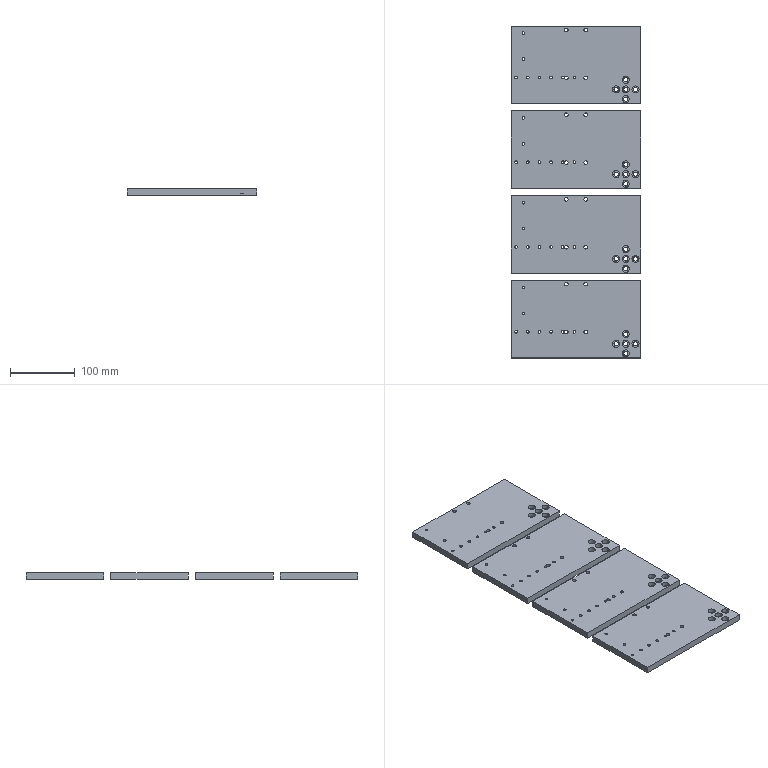CAM job | NX | 3-axis milling, drilling | part box 200 x 513 x 10 mm | stock box 205 x 518 x 10 mm
Tools:
number,name,description,diameter,corner_radius,flute_length,length,flutes
6,D6,平底铣刀-粗,6.0,0.0,25.0,75.0,2
9,D10,平底铣刀-粗,10.0,0.0,35.0,75.0,2
17,D3-J,平底铣刀-精,3.0,0.0,50.0,75.0,2
7,D6-J,平底铣刀-精,6.0,0.0,25.0,75.0,2
2,D6倒角刀,倒角刀,6.0,0.0,3.0,25.0,2
14,ZT4.2,钻头,4.2,0.0,35.0,50.0,2
17,ZT5.5,钻头,5.5,0.0,35.0,50.0,2
18,ZT6.6,钻头,6.6,0.0,35.0,50.0,2
Operations:
program,operation,operation_type,tool,method,geometry_group,spindle_rpm,surface_speed,feed_per_tooth,feed_cut,feed_plunge,cut_length_mm,path_length_mm,cut_time_min,machine_time_min
A,SPOT,Operation,D6倒角刀,METHOD,W-A,3000.0,56.549,0.0333,200.0,0.0,170.0,2343.871,0.85,1.067
A,DRILL,Operation,ZT4.2,METHOD,W-A,3000.0,38.924,0.0167,100.0,0.0,342.4,1713.674,3.424,3.561
A,DRILL_2,Operation,ZT5.5,METHOD,W-A,2600.0,44.925,0.0231,120.0,0.0,171.2,1104.587,1.427,1.52
A,DRILL_3,Operation,ZT6.6,METHOD,W-A,2500.0,51.836,0.03,150.0,0.0,214.0,1080.175,1.427,1.513
A,HOLEROUGH_1,CylinderMilling,D6,METHOD,W-A,6000.0,113.097,0.1667,2000.0,100.0,4737.362,6369.854,2.369,2.532
A,CONTOURROUGH_2,VolumeBased25DMillingOperation,D10,METHOD,W-A,6000.0,188.0,0.25,4000.0,80.0,56457.731,57435.075,14.114,14.212
A,HOLESIDE_1,CylinderMilling,D6-J,METHOD,W-A,6000.0,113.097,0.0667,800.0,100.0,433.835,2208.327,0.5423,0.7197
A,FLOORWALLHELIXFINISH-M_COPY,VolumeBased25DMillingOperation,D3-J,HELIXFINISH-DEPTHK-STEPG,W-A,8000.0,75.398,0.0312,500.0,100.0,3774.409,6069.896,7.549,7.778
A,FLOORWALLHELIXFINISH-M_COPY_COPY,VolumeBased25DMillingOperation,D3-J,HELIXFINISH-DEPTHK-STEPG,W-A,8000.0,75.398,0.0312,500.0,100.0,2952.803,4661.884,5.906,6.077
A,BODYONLY,SurfaceContour,D6倒角刀,METHOD,W-A,6000.0,113.0,0.125,1200.0,100.0,2629.259,3165.467,2.191,2.245
A,DRILLCHAMFER_1,Operation,D6倒角刀,METHOD,W-A,5000.0,94.248,0.015,150.0,0.0,181.344,1458.878,1.209,1.337
A,MILLCHAMFER_1,PlanarMilling,D6倒角刀,METHOD,W-A,6000.0,113.097,0.05,600.0,100.0,284.714,1669.792,0.4745,0.613
A,MILLCHAMFER_2,PlanarMilling,D6倒角刀,METHOD,W-A,6000.0,113.097,0.05,600.0,100.0,698.211,2204.59,1.164,1.314
A,CONTOURSEMI_2,VolumeBased25DMillingOperation,D6-J,METHOD,W-A,6000.0,113.0,0.0833,1000.0,100.0,2655.063,3476.519,2.655,2.737
A,CONTOURFINISH_2,VolumeBased25DMillingOperation,D6-J,METHOD,W-A,6000.0,113.0,0.0833,1000.0,100.0,2654.263,3477.951,2.654,2.737